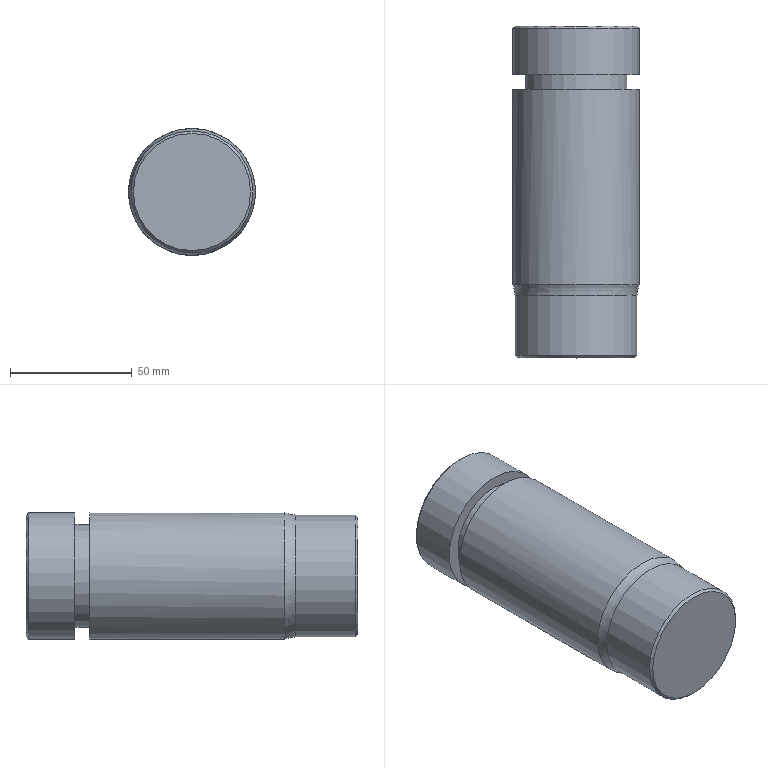Part | NX | features solid 2 | 1 solid | 11 faces | box 52 x 136 x 52 mm | volume 279657 mm3 | plane 4 | cylinder 4 | cone 2 | torus 1 | commonest cylinder face diameters 52 x2 42 x1 50 x1
STEP:
#1=CARTESIAN_POINT('',(935.,291.,59.));
#2=VERTEX_POINT('',#1);
#3=CARTESIAN_POINT('',(935.,291.,80.));
#4=DIRECTION('',(0.,-1.,0.));
#5=DIRECTION('',(0.,0.,-1.));
#6=AXIS2_PLACEMENT_3D('',#3,#4,#5);
#7=CIRCLE('',#6,21.);
#8=EDGE_CURVE('',#2,#2,#7,.T.);
#9=ORIENTED_EDGE('',*,*,#8,.F.);
#10=EDGE_LOOP('',(#9));
#11=FACE_BOUND('',#10,.T.);
#12=CARTESIAN_POINT('',(935.,291.,106.));
#13=VERTEX_POINT('',#12);
#14=CARTESIAN_POINT('',(935.,291.,80.));
#15=DIRECTION('',(0.,1.,0.));
#16=DIRECTION('',(0.,0.,1.));
#17=AXIS2_PLACEMENT_3D('',#14,#15,#16);
#18=CIRCLE('',#17,26.);
#19=EDGE_CURVE('',#13,#13,#18,.T.);
#20=ORIENTED_EDGE('',*,*,#19,.F.);
#21=EDGE_LOOP('',(#20));
#22=FACE_BOUND('',#21,.T.);
#23=CARTESIAN_POINT('',(935.,291.,80.));
#24=DIRECTION('',(0.,-1.,0.));
#25=DIRECTION('',(0.,0.,-1.));
#26=AXIS2_PLACEMENT_3D('',#23,#24,#25);
#27=PLANE('',#26);
#28=ADVANCED_FACE('',(#11,#22),#27,.T.);
#29=CARTESIAN_POINT('',(935.,311.,105.));
#30=VERTEX_POINT('',#29);
#31=CARTESIAN_POINT('',(935.,311.,80.));
#32=DIRECTION('',(0.,1.,0.));
#33=DIRECTION('',(0.,0.,1.));
#34=AXIS2_PLACEMENT_3D('',#31,#32,#33);
#35=CIRCLE('',#34,25.);
#36=EDGE_CURVE('',#30,#30,#35,.T.);
#37=ORIENTED_EDGE('',*,*,#36,.T.);
#38=EDGE_LOOP('',(#37));
#39=FACE_BOUND('',#38,.T.);
#40=CARTESIAN_POINT('',(935.,311.,80.));
#41=DIRECTION('',(0.,1.,0.));
#42=DIRECTION('',(0.,0.,1.));
#43=AXIS2_PLACEMENT_3D('',#40,#41,#42);
#44=PLANE('',#43);
#45=ADVANCED_FACE('',(#39),#44,.T.);
#46=CARTESIAN_POINT('',(935.,310.,106.));
#47=VERTEX_POINT('',#46);
#48=CARTESIAN_POINT('',(935.,310.,80.));
#49=DIRECTION('',(0.,1.,0.));
#50=DIRECTION('',(0.,0.,1.));
#51=AXIS2_PLACEMENT_3D('',#48,#49,#50);
#52=CIRCLE('',#51,26.);
#53=EDGE_CURVE('',#47,#47,#52,.F.);
#54=ORIENTED_EDGE('',*,*,#53,.T.);
#55=EDGE_LOOP('',(#54));
#56=FACE_BOUND('',#55,.T.);
#57=ORIENTED_EDGE('',*,*,#19,.T.);
#58=EDGE_LOOP('',(#57));
#59=FACE_BOUND('',#58,.T.);
#60=CARTESIAN_POINT('',(935.,311.,80.));
#61=DIRECTION('',(0.,-1.,0.));
#62=DIRECTION('',(0.,0.,-1.));
#63=AXIS2_PLACEMENT_3D('',#60,#61,#62);
#64=CYLINDRICAL_SURFACE('',#63,26.);
#65=ADVANCED_FACE('',(#56,#59),#64,.T.);
#66=CARTESIAN_POINT('',(935.,285.,101.));
#67=VERTEX_POINT('',#66);
#68=CARTESIAN_POINT('',(935.,285.,80.));
#69=DIRECTION('',(0.,1.,0.));
#70=DIRECTION('',(0.,0.,1.));
#71=AXIS2_PLACEMENT_3D('',#68,#69,#70);
#72=CIRCLE('',#71,21.);
#73=EDGE_CURVE('',#67,#67,#72,.F.);
#74=ORIENTED_EDGE('',*,*,#73,.F.);
#75=EDGE_LOOP('',(#74));
#76=FACE_BOUND('',#75,.T.);
#77=ORIENTED_EDGE('',*,*,#8,.T.);
#78=EDGE_LOOP('',(#77));
#79=FACE_BOUND('',#78,.T.);
#80=CARTESIAN_POINT('',(935.,291.,80.));
#81=DIRECTION('',(0.,-1.,0.));
#82=DIRECTION('',(0.,0.,-1.));
#83=AXIS2_PLACEMENT_3D('',#80,#81,#82);
#84=CYLINDRICAL_SURFACE('',#83,21.);
#85=ADVANCED_FACE('',(#76,#79),#84,.T.);
#86=ORIENTED_EDGE('',*,*,#73,.T.);
#87=EDGE_LOOP('',(#86));
#88=FACE_BOUND('',#87,.T.);
#89=CARTESIAN_POINT('',(935.,285.,54.));
#90=VERTEX_POINT('',#89);
#91=CARTESIAN_POINT('',(935.,285.,80.));
#92=DIRECTION('',(0.,-1.,0.));
#93=DIRECTION('',(0.,0.,-1.));
#94=AXIS2_PLACEMENT_3D('',#91,#92,#93);
#95=CIRCLE('',#94,26.);
#96=EDGE_CURVE('',#90,#90,#95,.T.);
#97=ORIENTED_EDGE('',*,*,#96,.F.);
#98=EDGE_LOOP('',(#97));
#99=FACE_BOUND('',#98,.T.);
#100=CARTESIAN_POINT('',(935.,285.,80.));
#101=DIRECTION('',(0.,1.,0.));
#102=DIRECTION('',(0.,0.,1.));
#103=AXIS2_PLACEMENT_3D('',#100,#101,#102);
#104=PLANE('',#103);
#105=ADVANCED_FACE('',(#88,#99),#104,.T.);
#106=CARTESIAN_POINT('',(935.,205.,106.));
#107=VERTEX_POINT('',#106);
#108=CARTESIAN_POINT('',(935.,205.,80.));
#109=DIRECTION('',(0.,1.,0.));
#110=DIRECTION('',(0.,0.,1.));
#111=AXIS2_PLACEMENT_3D('',#108,#109,#110);
#112=CIRCLE('',#111,26.);
#113=EDGE_CURVE('',#107,#107,#112,.T.);
#114=ORIENTED_EDGE('',*,*,#113,.T.);
#115=EDGE_LOOP('',(#114));
#116=FACE_BOUND('',#115,.T.);
#117=ORIENTED_EDGE('',*,*,#96,.T.);
#118=EDGE_LOOP('',(#117));
#119=FACE_BOUND('',#118,.T.);
#120=CARTESIAN_POINT('',(935.,285.,80.));
#121=DIRECTION('',(0.,-1.,0.));
#122=DIRECTION('',(0.,0.,-1.));
#123=AXIS2_PLACEMENT_3D('',#120,#121,#122);
#124=CYLINDRICAL_SURFACE('',#123,26.);
#125=ADVANCED_FACE('',(#116,#119),#124,.T.);
#126=CARTESIAN_POINT('',(935.,175.,56.));
#127=VERTEX_POINT('',#126);
#128=CARTESIAN_POINT('',(935.,175.,80.));
#129=DIRECTION('',(0.,-1.,0.));
#130=DIRECTION('',(0.,0.,-1.));
#131=AXIS2_PLACEMENT_3D('',#128,#129,#130);
#132=CIRCLE('',#131,24.);
#133=EDGE_CURVE('',#127,#127,#132,.T.);
#134=ORIENTED_EDGE('',*,*,#133,.T.);
#135=EDGE_LOOP('',(#134));
#136=FACE_BOUND('',#135,.T.);
#137=CARTESIAN_POINT('',(935.,175.,80.));
#138=DIRECTION('',(0.,-1.,0.));
#139=DIRECTION('',(0.,0.,-1.));
#140=AXIS2_PLACEMENT_3D('',#137,#138,#139);
#141=PLANE('',#140);
#142=ADVANCED_FACE('',(#136),#141,.T.);
#143=CARTESIAN_POINT('',(935.,176.,55.));
#144=VERTEX_POINT('',#143);
#145=CARTESIAN_POINT('',(935.,176.,80.));
#146=DIRECTION('',(0.,-1.,0.));
#147=DIRECTION('',(0.,0.,-1.));
#148=AXIS2_PLACEMENT_3D('',#145,#146,#147);
#149=CIRCLE('',#148,25.);
#150=EDGE_CURVE('',#144,#144,#149,.F.);
#151=ORIENTED_EDGE('',*,*,#150,.T.);
#152=EDGE_LOOP('',(#151));
#153=FACE_BOUND('',#152,.T.);
#154=CARTESIAN_POINT('',(935.,200.641,105.));
#155=VERTEX_POINT('',#154);
#156=CARTESIAN_POINT('',(935.,200.641,80.));
#157=DIRECTION('',(0.,1.,0.));
#158=DIRECTION('',(0.,0.,1.));
#159=AXIS2_PLACEMENT_3D('',#156,#157,#158);
#160=CIRCLE('',#159,25.);
#161=EDGE_CURVE('',#155,#155,#160,.F.);
#162=ORIENTED_EDGE('',*,*,#161,.T.);
#163=EDGE_LOOP('',(#162));
#164=FACE_BOUND('',#163,.T.);
#165=CARTESIAN_POINT('',(935.,205.,80.));
#166=DIRECTION('',(0.,-1.,0.));
#167=DIRECTION('',(0.,0.,-1.));
#168=AXIS2_PLACEMENT_3D('',#165,#166,#167);
#169=CYLINDRICAL_SURFACE('',#168,25.);
#170=ADVANCED_FACE('',(#153,#164),#169,.T.);
#171=ORIENTED_EDGE('',*,*,#36,.F.);
#172=EDGE_LOOP('',(#171));
#173=FACE_BOUND('',#172,.T.);
#174=ORIENTED_EDGE('',*,*,#53,.F.);
#175=EDGE_LOOP('',(#174));
#176=FACE_BOUND('',#175,.T.);
#177=CARTESIAN_POINT('',(935.,310.,80.));
#178=DIRECTION('',(0.,-1.,0.));
#179=DIRECTION('',(0.,0.,-1.));
#180=AXIS2_PLACEMENT_3D('',#177,#178,#179);
#181=CONICAL_SURFACE('',#180,26.,0.7854);
#182=ADVANCED_FACE('',(#173,#176),#181,.T.);
#183=ORIENTED_EDGE('',*,*,#113,.F.);
#184=EDGE_LOOP('',(#183));
#185=FACE_BOUND('',#184,.T.);
#186=ORIENTED_EDGE('',*,*,#161,.F.);
#187=EDGE_LOOP('',(#186));
#188=FACE_BOUND('',#187,.T.);
#189=CARTESIAN_POINT('',(935.,200.641,80.));
#190=DIRECTION('',(0.,1.,0.));
#191=DIRECTION('',(0.,0.,1.));
#192=AXIS2_PLACEMENT_3D('',#189,#190,#191);
#193=TOROIDAL_SURFACE('',#192,35.,10.);
#194=ADVANCED_FACE('',(#185,#188),#193,.F.);
#195=ORIENTED_EDGE('',*,*,#133,.F.);
#196=EDGE_LOOP('',(#195));
#197=FACE_BOUND('',#196,.T.);
#198=ORIENTED_EDGE('',*,*,#150,.F.);
#199=EDGE_LOOP('',(#198));
#200=FACE_BOUND('',#199,.T.);
#201=CARTESIAN_POINT('',(935.,176.,80.));
#202=DIRECTION('',(0.,1.,0.));
#203=DIRECTION('',(0.,0.,1.));
#204=AXIS2_PLACEMENT_3D('',#201,#202,#203);
#205=CONICAL_SURFACE('',#204,25.,0.7854);
#206=ADVANCED_FACE('',(#197,#200),#205,.T.);
#207=CLOSED_SHELL('',(#28,#45,#65,#85,#105,#125,#142,#170,#182,#194,#206));
#208=MANIFOLD_SOLID_BREP('',#207);
#209=(LENGTH_UNIT()NAMED_UNIT(*)SI_UNIT(.MILLI.,.METRE.));
#210=UNCERTAINTY_MEASURE_WITH_UNIT(LENGTH_MEASURE(0.00001),#209,'','');
#211=(NAMED_UNIT(*)PLANE_ANGLE_UNIT()SI_UNIT($,.RADIAN.));
#212=(NAMED_UNIT(*)SI_UNIT($,.STERADIAN.)SOLID_ANGLE_UNIT());
#213=(GEOMETRIC_REPRESENTATION_CONTEXT(3)GLOBAL_UNCERTAINTY_ASSIGNED_CONTEXT((#210))GLOBAL_UNIT_ASSIGNED_CONTEXT((#209,#211,#212))REPRESENTATION_CONTEXT('',''));
#214=ADVANCED_BREP_SHAPE_REPRESENTATION('',(#208),#213);